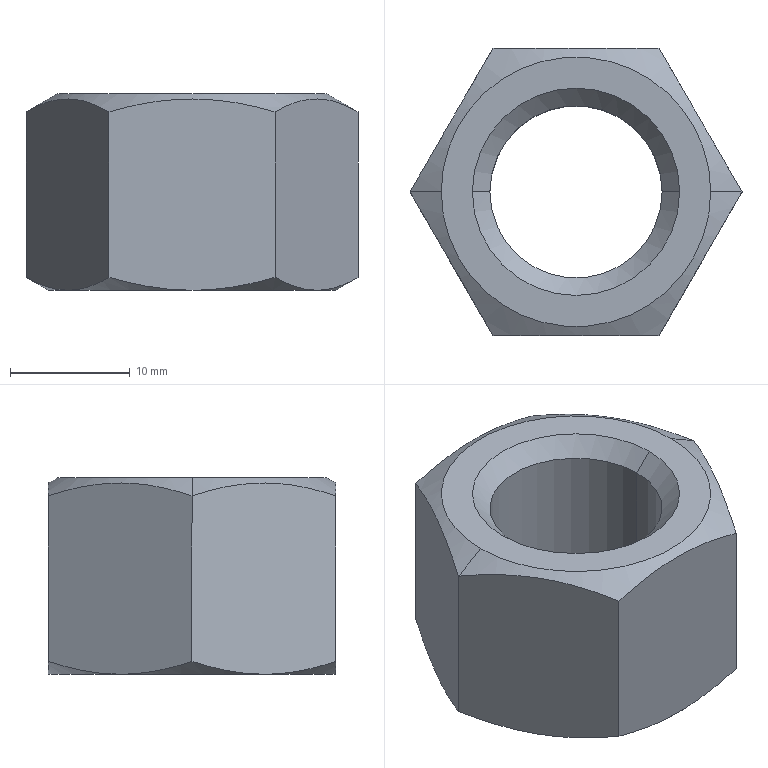Part | STEP file | Hex Nut GB 6170-2000 M16(X1.5)_GB_HEXAGON_TYPE10 M16X1.5-N | 1 solid | 23 faces | box 27.713 x 24 x 16.4 mm | volume 5375 mm3 | cone 13 | plane 8 | cylinder 2 | commonest cylinder face diameters 14.376 x2